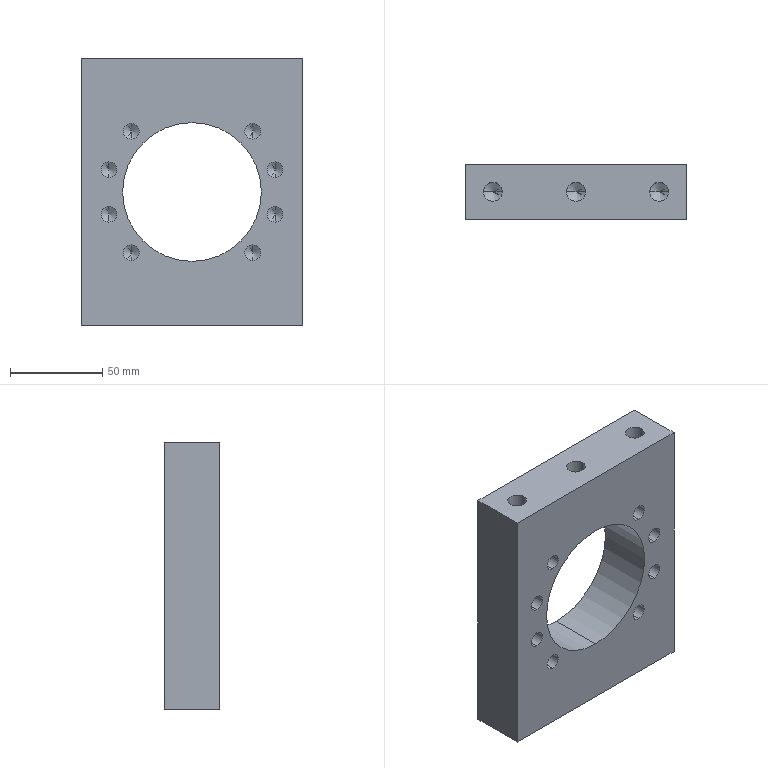Part | SolidWorks | features HoleWzd 2, Extrusion 1, MirrorPattern 1 | 1 solid | 64 faces | box 120 x 30 x 145 mm | volume 363114 mm3 | cylinder 30 | cone 28 | plane 6 | commonest cylinder face diameters 8.5 x16 10.2 x12 75 x2